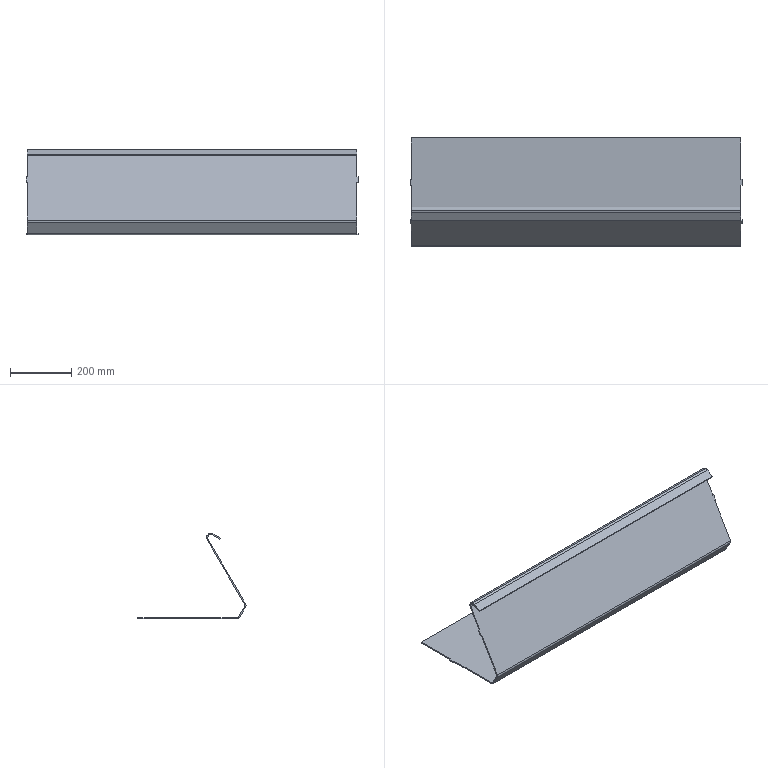Part | SolidWorks | features SM3dBend 3, FlatPattern 1, SMBaseFlange 1, SheetMetal 1 | 1 solid | 48 faces | box 1084 x 353.006 x 279.006 mm | volume 2939163 mm3 | plane 40 | cylinder 8 | commonest cylinder face diameters 10 x2 18 x2 20 x2 28 x2
STEP:
#1=CARTESIAN_POINT('',(1271.731,577.865,275.006));
#2=VERTEX_POINT('',#1);
#3=CARTESIAN_POINT('',(1271.731,570.865,273.13));
#4=VERTEX_POINT('',#3);
#5=CARTESIAN_POINT('',(1271.731,577.865,261.006));
#6=DIRECTION('',(1.,0.,0.));
#7=DIRECTION('',(0.,0.,1.));
#8=AXIS2_PLACEMENT_3D('',#5,#6,#7);
#9=CIRCLE('',#8,14.);
#10=EDGE_CURVE('',#2,#4,#9,.T.);
#11=ORIENTED_EDGE('',*,*,#10,.F.);
#12=CARTESIAN_POINT('',(195.731,577.865,275.006));
#13=VERTEX_POINT('',#12);
#14=CARTESIAN_POINT('',(1810.249,577.865,275.006));
#15=DIRECTION('',(-1.,0.,0.));
#16=VECTOR('',#15,1000.);
#17=LINE('',#14,#16);
#18=EDGE_CURVE('',#2,#13,#17,.T.);
#19=ORIENTED_EDGE('',*,*,#18,.T.);
#20=CARTESIAN_POINT('',(195.731,570.865,273.13));
#21=VERTEX_POINT('',#20);
#22=CARTESIAN_POINT('',(195.731,577.865,261.006));
#23=DIRECTION('',(-1.,0.,0.));
#24=DIRECTION('',(0.,0.,1.));
#25=AXIS2_PLACEMENT_3D('',#22,#23,#24);
#26=CIRCLE('',#25,14.);
#27=EDGE_CURVE('',#21,#13,#26,.T.);
#28=ORIENTED_EDGE('',*,*,#27,.F.);
#29=CARTESIAN_POINT('',(0.,570.865,273.13));
#30=DIRECTION('',(1.,0.,0.));
#31=VECTOR('',#30,1000.);
#32=LINE('',#29,#31);
#33=EDGE_CURVE('',#21,#4,#32,.T.);
#34=ORIENTED_EDGE('',*,*,#33,.T.);
#35=EDGE_LOOP('',(#11,#19,#28,#34));
#36=FACE_OUTER_BOUND('',#35,.T.);
#37=CARTESIAN_POINT('',(1810.249,577.865,261.006));
#38=DIRECTION('',(-1.,0.,0.));
#39=DIRECTION('',(0.,0.,1.));
#40=AXIS2_PLACEMENT_3D('',#37,#38,#39);
#41=CYLINDRICAL_SURFACE('',#40,14.);
#42=ADVANCED_FACE('',(#36),#41,.T.);
#43=CARTESIAN_POINT('',(1271.731,586.525,256.006));
#44=VERTEX_POINT('',#43);
#45=CARTESIAN_POINT('',(1271.731,577.865,271.006));
#46=VERTEX_POINT('',#45);
#47=CARTESIAN_POINT('',(1271.731,577.865,261.006));
#48=DIRECTION('',(1.,0.,0.));
#49=DIRECTION('',(0.,0.,1.));
#50=AXIS2_PLACEMENT_3D('',#47,#48,#49);
#51=CIRCLE('',#50,10.);
#52=EDGE_CURVE('',#44,#46,#51,.T.);
#53=ORIENTED_EDGE('',*,*,#52,.T.);
#54=CARTESIAN_POINT('',(195.731,577.865,271.006));
#55=VERTEX_POINT('',#54);
#56=CARTESIAN_POINT('',(1810.249,577.865,271.006));
#57=DIRECTION('',(-1.,0.,0.));
#58=VECTOR('',#57,1000.);
#59=LINE('',#56,#58);
#60=EDGE_CURVE('',#46,#55,#59,.T.);
#61=ORIENTED_EDGE('',*,*,#60,.T.);
#62=CARTESIAN_POINT('',(195.731,586.525,256.006));
#63=VERTEX_POINT('',#62);
#64=CARTESIAN_POINT('',(195.731,577.865,261.006));
#65=DIRECTION('',(-1.,0.,0.));
#66=DIRECTION('',(0.,0.,-1.));
#67=AXIS2_PLACEMENT_3D('',#64,#65,#66);
#68=CIRCLE('',#67,10.);
#69=EDGE_CURVE('',#55,#63,#68,.T.);
#70=ORIENTED_EDGE('',*,*,#69,.T.);
#71=CARTESIAN_POINT('',(0.,586.525,256.006));
#72=DIRECTION('',(1.,0.,0.));
#73=VECTOR('',#72,1000.);
#74=LINE('',#71,#73);
#75=EDGE_CURVE('',#63,#44,#74,.T.);
#76=ORIENTED_EDGE('',*,*,#75,.T.);
#77=EDGE_LOOP('',(#53,#61,#70,#76));
#78=FACE_OUTER_BOUND('',#77,.T.);
#79=CARTESIAN_POINT('',(1810.249,577.865,261.006));
#80=DIRECTION('',(-1.,0.,0.));
#81=DIRECTION('',(0.,0.,1.));
#82=AXIS2_PLACEMENT_3D('',#79,#80,#81);
#83=CYLINDRICAL_SURFACE('',#82,10.);
#84=ADVANCED_FACE('',(#78),#83,.F.);
#85=CARTESIAN_POINT('',(195.731,548.991,182.994));
#86=VERTEX_POINT('',#85);
#87=CARTESIAN_POINT('',(195.731,589.989,254.006));
#88=VERTEX_POINT('',#87);
#89=CARTESIAN_POINT('',(195.731,618.751,303.822));
#90=DIRECTION('',(0.,0.5,0.866));
#91=VECTOR('',#90,1000.);
#92=LINE('',#89,#91);
#93=EDGE_CURVE('',#86,#88,#92,.T.);
#94=ORIENTED_EDGE('',*,*,#93,.T.);
#95=CARTESIAN_POINT('',(1271.731,589.989,254.006));
#96=VERTEX_POINT('',#95);
#97=CARTESIAN_POINT('',(0.,589.989,254.006));
#98=DIRECTION('',(1.,0.,0.));
#99=VECTOR('',#98,1000.);
#100=LINE('',#97,#99);
#101=EDGE_CURVE('',#88,#96,#100,.T.);
#102=ORIENTED_EDGE('',*,*,#101,.T.);
#103=CARTESIAN_POINT('',(1271.731,548.991,182.994));
#104=VERTEX_POINT('',#103);
#105=CARTESIAN_POINT('',(1271.731,618.751,303.822));
#106=DIRECTION('',(0.,-0.5,-0.866));
#107=VECTOR('',#106,1000.);
#108=LINE('',#105,#107);
#109=EDGE_CURVE('',#96,#104,#108,.T.);
#110=ORIENTED_EDGE('',*,*,#109,.T.);
#111=CARTESIAN_POINT('',(1275.731,548.991,182.994));
#112=VERTEX_POINT('',#111);
#113=CARTESIAN_POINT('',(1275.731,548.991,182.994));
#114=DIRECTION('',(1.,0.,0.));
#115=VECTOR('',#114,1000.);
#116=LINE('',#113,#115);
#117=EDGE_CURVE('',#104,#112,#116,.T.);
#118=ORIENTED_EDGE('',*,*,#117,.T.);
#119=CARTESIAN_POINT('',(1275.731,538.991,165.674));
#120=VERTEX_POINT('',#119);
#121=CARTESIAN_POINT('',(1275.731,538.991,165.674));
#122=DIRECTION('',(0.,-0.5,-0.866));
#123=VECTOR('',#122,1000.);
#124=LINE('',#121,#123);
#125=EDGE_CURVE('',#112,#120,#124,.T.);
#126=ORIENTED_EDGE('',*,*,#125,.T.);
#127=CARTESIAN_POINT('',(1271.731,538.991,165.674));
#128=VERTEX_POINT('',#127);
#129=CARTESIAN_POINT('',(1275.731,538.991,165.674));
#130=DIRECTION('',(-1.,0.,0.));
#131=VECTOR('',#130,1000.);
#132=LINE('',#129,#131);
#133=EDGE_CURVE('',#120,#128,#132,.T.);
#134=ORIENTED_EDGE('',*,*,#133,.T.);
#135=CARTESIAN_POINT('',(1271.731,467.476,41.807));
#136=VERTEX_POINT('',#135);
#137=CARTESIAN_POINT('',(1271.731,538.991,165.674));
#138=DIRECTION('',(0.,-0.5,-0.866));
#139=VECTOR('',#138,1000.);
#140=LINE('',#137,#139);
#141=EDGE_CURVE('',#128,#136,#140,.T.);
#142=ORIENTED_EDGE('',*,*,#141,.T.);
#143=CARTESIAN_POINT('',(195.731,467.476,41.807));
#144=VERTEX_POINT('',#143);
#145=CARTESIAN_POINT('',(0.,467.476,41.807));
#146=DIRECTION('',(1.,0.,0.));
#147=VECTOR('',#146,1000.);
#148=LINE('',#145,#147);
#149=EDGE_CURVE('',#144,#136,#148,.T.);
#150=ORIENTED_EDGE('',*,*,#149,.F.);
#151=CARTESIAN_POINT('',(195.731,538.991,165.674));
#152=VERTEX_POINT('',#151);
#153=CARTESIAN_POINT('',(195.731,538.991,165.674));
#154=DIRECTION('',(0.,0.5,0.866));
#155=VECTOR('',#154,1000.);
#156=LINE('',#153,#155);
#157=EDGE_CURVE('',#144,#152,#156,.T.);
#158=ORIENTED_EDGE('',*,*,#157,.T.);
#159=CARTESIAN_POINT('',(191.731,538.991,165.674));
#160=VERTEX_POINT('',#159);
#161=CARTESIAN_POINT('',(191.731,538.991,165.674));
#162=DIRECTION('',(-1.,0.,0.));
#163=VECTOR('',#162,1000.);
#164=LINE('',#161,#163);
#165=EDGE_CURVE('',#152,#160,#164,.T.);
#166=ORIENTED_EDGE('',*,*,#165,.T.);
#167=CARTESIAN_POINT('',(191.731,548.991,182.994));
#168=VERTEX_POINT('',#167);
#169=CARTESIAN_POINT('',(191.731,548.991,182.994));
#170=DIRECTION('',(0.,0.5,0.866));
#171=VECTOR('',#170,1000.);
#172=LINE('',#169,#171);
#173=EDGE_CURVE('',#160,#168,#172,.T.);
#174=ORIENTED_EDGE('',*,*,#173,.T.);
#175=CARTESIAN_POINT('',(191.731,548.991,182.994));
#176=DIRECTION('',(1.,0.,0.));
#177=VECTOR('',#176,1000.);
#178=LINE('',#175,#177);
#179=EDGE_CURVE('',#168,#86,#178,.T.);
#180=ORIENTED_EDGE('',*,*,#179,.T.);
#181=EDGE_LOOP('',(#94,#102,#110,#118,#126,#134,#142,#150,#158,#166,#174,#180));
#182=FACE_OUTER_BOUND('',#181,.T.);
#183=CARTESIAN_POINT('',(0.,686.774,421.641));
#184=DIRECTION('',(0.,-0.866,0.5));
#185=DIRECTION('',(-1.,0.,0.));
#186=AXIS2_PLACEMENT_3D('',#183,#184,#185);
#187=PLANE('',#186);
#188=ADVANCED_FACE('',(#182),#187,.F.);
#189=CARTESIAN_POINT('',(195.731,487.283,2.5));
#190=VERTEX_POINT('',#189);
#191=CARTESIAN_POINT('',(195.731,467.476,36.807));
#192=VERTEX_POINT('',#191);
#193=CARTESIAN_POINT('',(195.731,392.611,166.478));
#194=DIRECTION('',(0.,-0.5,0.866));
#195=VECTOR('',#194,1000.);
#196=LINE('',#193,#195);
#197=EDGE_CURVE('',#190,#192,#196,.T.);
#198=ORIENTED_EDGE('',*,*,#197,.T.);
#199=CARTESIAN_POINT('',(1271.731,467.476,36.807));
#200=VERTEX_POINT('',#199);
#201=CARTESIAN_POINT('',(0.,467.476,36.807));
#202=DIRECTION('',(1.,0.,0.));
#203=VECTOR('',#202,1000.);
#204=LINE('',#201,#203);
#205=EDGE_CURVE('',#192,#200,#204,.T.);
#206=ORIENTED_EDGE('',*,*,#205,.T.);
#207=CARTESIAN_POINT('',(1271.731,487.283,2.5));
#208=VERTEX_POINT('',#207);
#209=CARTESIAN_POINT('',(1271.731,392.611,166.478));
#210=DIRECTION('',(0.,0.5,-0.866));
#211=VECTOR('',#210,1000.);
#212=LINE('',#209,#211);
#213=EDGE_CURVE('',#200,#208,#212,.T.);
#214=ORIENTED_EDGE('',*,*,#213,.T.);
#215=CARTESIAN_POINT('',(0.,487.283,2.5));
#216=DIRECTION('',(1.,0.,0.));
#217=VECTOR('',#216,1000.);
#218=LINE('',#215,#217);
#219=EDGE_CURVE('',#190,#208,#218,.T.);
#220=ORIENTED_EDGE('',*,*,#219,.F.);
#221=EDGE_LOOP('',(#198,#206,#214,#220));
#222=FACE_OUTER_BOUND('',#221,.T.);
#223=CARTESIAN_POINT('',(0.,244.828,422.446));
#224=DIRECTION('',(0.,-0.866,-0.5));
#225=DIRECTION('',(-1.,0.,0.));
#226=AXIS2_PLACEMENT_3D('',#223,#224,#225);
#227=PLANE('',#226);
#228=ADVANCED_FACE('',(#222),#227,.F.);
#229=CARTESIAN_POINT('',(195.731,464.012,34.807));
#230=VERTEX_POINT('',#229);
#231=CARTESIAN_POINT('',(195.731,464.012,34.807));
#232=DIRECTION('',(0.,-0.866,-0.5));
#233=VECTOR('',#232,1000.);
#234=LINE('',#231,#233);
#235=EDGE_CURVE('',#192,#230,#234,.T.);
#236=ORIENTED_EDGE('',*,*,#235,.F.);
#237=ORIENTED_EDGE('',*,*,#197,.F.);
#238=CARTESIAN_POINT('',(195.731,483.819,0.5));
#239=VERTEX_POINT('',#238);
#240=CARTESIAN_POINT('',(195.731,483.819,0.5));
#241=DIRECTION('',(0.,-0.866,-0.5));
#242=VECTOR('',#241,1000.);
#243=LINE('',#240,#242);
#244=EDGE_CURVE('',#190,#239,#243,.T.);
#245=ORIENTED_EDGE('',*,*,#244,.T.);
#246=CARTESIAN_POINT('',(195.731,389.147,164.478));
#247=DIRECTION('',(0.,-0.5,0.866));
#248=VECTOR('',#247,1000.);
#249=LINE('',#246,#248);
#250=EDGE_CURVE('',#239,#230,#249,.T.);
#251=ORIENTED_EDGE('',*,*,#250,.T.);
#252=EDGE_LOOP('',(#236,#237,#245,#251));
#253=FACE_OUTER_BOUND('',#252,.T.);
#254=CARTESIAN_POINT('',(195.731,389.147,164.478));
#255=DIRECTION('',(-1.,0.,0.));
#256=DIRECTION('',(0.,0.866,0.5));
#257=AXIS2_PLACEMENT_3D('',#254,#255,#256);
#258=PLANE('',#257);
#259=ADVANCED_FACE('',(#253),#258,.T.);
#260=CARTESIAN_POINT('',(1271.731,464.012,34.807));
#261=VERTEX_POINT('',#260);
#262=CARTESIAN_POINT('',(1271.731,464.012,34.807));
#263=DIRECTION('',(0.,0.866,0.5));
#264=VECTOR('',#263,1000.);
#265=LINE('',#262,#264);
#266=EDGE_CURVE('',#261,#200,#265,.T.);
#267=ORIENTED_EDGE('',*,*,#266,.F.);
#268=CARTESIAN_POINT('',(1271.731,483.819,0.5));
#269=VERTEX_POINT('',#268);
#270=CARTESIAN_POINT('',(1271.731,389.147,164.478));
#271=DIRECTION('',(0.,0.5,-0.866));
#272=VECTOR('',#271,1000.);
#273=LINE('',#270,#272);
#274=EDGE_CURVE('',#261,#269,#273,.T.);
#275=ORIENTED_EDGE('',*,*,#274,.T.);
#276=CARTESIAN_POINT('',(1271.731,483.819,0.5));
#277=DIRECTION('',(0.,0.866,0.5));
#278=VECTOR('',#277,1000.);
#279=LINE('',#276,#278);
#280=EDGE_CURVE('',#269,#208,#279,.T.);
#281=ORIENTED_EDGE('',*,*,#280,.T.);
#282=ORIENTED_EDGE('',*,*,#213,.F.);
#283=EDGE_LOOP('',(#267,#275,#281,#282));
#284=FACE_OUTER_BOUND('',#283,.T.);
#285=CARTESIAN_POINT('',(1271.731,389.147,164.478));
#286=DIRECTION('',(1.,0.,0.));
#287=DIRECTION('',(0.,-0.866,-0.5));
#288=AXIS2_PLACEMENT_3D('',#285,#286,#287);
#289=PLANE('',#288);
#290=ADVANCED_FACE('',(#284),#289,.T.);
#291=CARTESIAN_POINT('',(0.,464.012,34.807));
#292=DIRECTION('',(1.,0.,0.));
#293=VECTOR('',#292,1000.);
#294=LINE('',#291,#293);
#295=EDGE_CURVE('',#230,#261,#294,.T.);
#296=ORIENTED_EDGE('',*,*,#295,.F.);
#297=ORIENTED_EDGE('',*,*,#250,.F.);
#298=CARTESIAN_POINT('',(0.,483.819,0.5));
#299=DIRECTION('',(1.,0.,0.));
#300=VECTOR('',#299,1000.);
#301=LINE('',#298,#300);
#302=EDGE_CURVE('',#239,#269,#301,.T.);
#303=ORIENTED_EDGE('',*,*,#302,.T.);
#304=ORIENTED_EDGE('',*,*,#274,.F.);
#305=EDGE_LOOP('',(#296,#297,#303,#304));
#306=FACE_OUTER_BOUND('',#305,.T.);
#307=CARTESIAN_POINT('',(0.,241.363,420.446));
#308=DIRECTION('',(0.,-0.866,-0.5));
#309=DIRECTION('',(-1.,0.,0.));
#310=AXIS2_PLACEMENT_3D('',#307,#308,#309);
#311=PLANE('',#310);
#312=ADVANCED_FACE('',(#306),#311,.T.);
#313=CARTESIAN_POINT('',(1271.731,660.806,0.));
#314=VERTEX_POINT('',#313);
#315=CARTESIAN_POINT('',(1275.731,660.806,0.));
#316=VERTEX_POINT('',#315);
#317=CARTESIAN_POINT('',(1275.731,660.806,0.));
#318=DIRECTION('',(1.,0.,0.));
#319=VECTOR('',#318,1000.);
#320=LINE('',#317,#319);
#321=EDGE_CURVE('',#314,#316,#320,.T.);
#322=ORIENTED_EDGE('',*,*,#321,.F.);
#323=CARTESIAN_POINT('',(1271.731,660.806,-4.));
#324=VERTEX_POINT('',#323);
#325=CARTESIAN_POINT('',(1271.731,660.806,-4.));
#326=DIRECTION('',(0.,0.,1.));
#327=VECTOR('',#326,1000.);
#328=LINE('',#325,#327);
#329=EDGE_CURVE('',#324,#314,#328,.T.);
#330=ORIENTED_EDGE('',*,*,#329,.F.);
#331=CARTESIAN_POINT('',(1275.731,660.806,-4.));
#332=VERTEX_POINT('',#331);
#333=CARTESIAN_POINT('',(1275.731,660.806,-4.));
#334=DIRECTION('',(1.,0.,0.));
#335=VECTOR('',#334,1000.);
#336=LINE('',#333,#335);
#337=EDGE_CURVE('',#324,#332,#336,.T.);
#338=ORIENTED_EDGE('',*,*,#337,.T.);
#339=CARTESIAN_POINT('',(1275.731,660.806,-4.));
#340=DIRECTION('',(0.,0.,1.));
#341=VECTOR('',#340,1000.);
#342=LINE('',#339,#341);
#343=EDGE_CURVE('',#332,#316,#342,.T.);
#344=ORIENTED_EDGE('',*,*,#343,.T.);
#345=EDGE_LOOP('',(#322,#330,#338,#344));
#346=FACE_OUTER_BOUND('',#345,.T.);
#347=CARTESIAN_POINT('',(1275.731,660.806,-4.));
#348=DIRECTION('',(0.,-1.,0.));
#349=DIRECTION('',(0.,0.,-1.));
#350=AXIS2_PLACEMENT_3D('',#347,#348,#349);
#351=PLANE('',#350);
#352=ADVANCED_FACE('',(#346),#351,.T.);
#353=CARTESIAN_POINT('',(1275.731,680.806,0.));
#354=VERTEX_POINT('',#353);
#355=CARTESIAN_POINT('',(1275.731,680.806,0.));
#356=DIRECTION('',(0.,1.,0.));
#357=VECTOR('',#356,1000.);
#358=LINE('',#355,#357);
#359=EDGE_CURVE('',#316,#354,#358,.T.);
#360=ORIENTED_EDGE('',*,*,#359,.F.);
#361=ORIENTED_EDGE('',*,*,#343,.F.);
#362=CARTESIAN_POINT('',(1275.731,680.806,-4.));
#363=VERTEX_POINT('',#362);
#364=CARTESIAN_POINT('',(1275.731,680.806,-4.));
#365=DIRECTION('',(0.,1.,0.));
#366=VECTOR('',#365,1000.);
#367=LINE('',#364,#366);
#368=EDGE_CURVE('',#332,#363,#367,.T.);
#369=ORIENTED_EDGE('',*,*,#368,.T.);
#370=CARTESIAN_POINT('',(1275.731,680.806,-4.));
#371=DIRECTION('',(0.,0.,1.));
#372=VECTOR('',#371,1000.);
#373=LINE('',#370,#372);
#374=EDGE_CURVE('',#363,#354,#373,.T.);
#375=ORIENTED_EDGE('',*,*,#374,.T.);
#376=EDGE_LOOP('',(#360,#361,#369,#375));
#377=FACE_OUTER_BOUND('',#376,.T.);
#378=CARTESIAN_POINT('',(1275.731,680.806,-4.));
#379=DIRECTION('',(1.,0.,0.));
#380=DIRECTION('',(0.,0.,-1.));
#381=AXIS2_PLACEMENT_3D('',#378,#379,#380);
#382=PLANE('',#381);
#383=ADVANCED_FACE('',(#377),#382,.T.);
#384=CARTESIAN_POINT('',(1271.731,680.806,0.));
#385=VERTEX_POINT('',#384);
#386=CARTESIAN_POINT('',(1275.731,680.806,0.));
#387=DIRECTION('',(-1.,0.,0.));
#388=VECTOR('',#387,1000.);
#389=LINE('',#386,#388);
#390=EDGE_CURVE('',#354,#385,#389,.T.);
#391=ORIENTED_EDGE('',*,*,#390,.F.);
#392=ORIENTED_EDGE('',*,*,#374,.F.);
#393=CARTESIAN_POINT('',(1271.731,680.806,-4.));
#394=VERTEX_POINT('',#393);
#395=CARTESIAN_POINT('',(1275.731,680.806,-4.));
#396=DIRECTION('',(-1.,0.,0.));
#397=VECTOR('',#396,1000.);
#398=LINE('',#395,#397);
#399=EDGE_CURVE('',#363,#394,#398,.T.);
#400=ORIENTED_EDGE('',*,*,#399,.T.);
#401=CARTESIAN_POINT('',(1271.731,680.806,-4.));
#402=DIRECTION('',(0.,0.,1.));
#403=VECTOR('',#402,1000.);
#404=LINE('',#401,#403);
#405=EDGE_CURVE('',#394,#385,#404,.T.);
#406=ORIENTED_EDGE('',*,*,#405,.T.);
#407=EDGE_LOOP('',(#391,#392,#400,#406));
#408=FACE_OUTER_BOUND('',#407,.T.);
#409=CARTESIAN_POINT('',(1275.731,680.806,-4.));
#410=DIRECTION('',(0.,1.,0.));
#411=DIRECTION('',(0.,0.,1.));
#412=AXIS2_PLACEMENT_3D('',#409,#410,#411);
#413=PLANE('',#412);
#414=ADVANCED_FACE('',(#408),#413,.T.);
#415=CARTESIAN_POINT('',(1271.731,815.812,0.));
#416=VERTEX_POINT('',#415);
#417=CARTESIAN_POINT('',(1271.731,680.806,0.));
#418=DIRECTION('',(0.,1.,0.));
#419=VECTOR('',#418,1000.);
#420=LINE('',#417,#419);
#421=EDGE_CURVE('',#385,#416,#420,.T.);
#422=ORIENTED_EDGE('',*,*,#421,.F.);
#423=ORIENTED_EDGE('',*,*,#405,.F.);
#424=CARTESIAN_POINT('',(1271.731,815.812,-4.));
#425=VERTEX_POINT('',#424);
#426=CARTESIAN_POINT('',(1271.731,680.806,-4.));
#427=DIRECTION('',(0.,1.,0.));
#428=VECTOR('',#427,1000.);
#429=LINE('',#426,#428);
#430=EDGE_CURVE('',#394,#425,#429,.T.);
#431=ORIENTED_EDGE('',*,*,#430,.T.);
#432=CARTESIAN_POINT('',(1271.731,815.812,-4.));
#433=DIRECTION('',(0.,0.,1.));
#434=VECTOR('',#433,1000.);
#435=LINE('',#432,#434);
#436=EDGE_CURVE('',#425,#416,#435,.T.);
#437=ORIENTED_EDGE('',*,*,#436,.T.);
#438=EDGE_LOOP('',(#422,#423,#431,#437));
#439=FACE_OUTER_BOUND('',#438,.T.);
#440=CARTESIAN_POINT('',(1271.731,680.806,-4.));
#441=DIRECTION('',(1.,0.,0.));
#442=DIRECTION('',(0.,0.,-1.));
#443=AXIS2_PLACEMENT_3D('',#440,#441,#442);
#444=PLANE('',#443);
#445=ADVANCED_FACE('',(#439),#444,.T.);
#446=CARTESIAN_POINT('',(195.731,815.812,0.));
#447=VERTEX_POINT('',#446);
#448=CARTESIAN_POINT('',(1271.731,815.812,0.));
#449=DIRECTION('',(-1.,0.,0.));
#450=VECTOR('',#449,1000.);
#451=LINE('',#448,#450);
#452=EDGE_CURVE('',#416,#447,#451,.T.);
#453=ORIENTED_EDGE('',*,*,#452,.F.);
#454=ORIENTED_EDGE('',*,*,#436,.F.);
#455=CARTESIAN_POINT('',(195.731,815.812,-4.));
#456=VERTEX_POINT('',#455);
#457=CARTESIAN_POINT('',(1271.731,815.812,-4.));
#458=DIRECTION('',(-1.,0.,0.));
#459=VECTOR('',#458,1000.);
#460=LINE('',#457,#459);
#461=EDGE_CURVE('',#425,#456,#460,.T.);
#462=ORIENTED_EDGE('',*,*,#461,.T.);
#463=CARTESIAN_POINT('',(195.731,815.812,-4.));
#464=DIRECTION('',(0.,0.,1.));
#465=VECTOR('',#464,1000.);
#466=LINE('',#463,#465);
#467=EDGE_CURVE('',#456,#447,#466,.T.);
#468=ORIENTED_EDGE('',*,*,#467,.T.);
#469=EDGE_LOOP('',(#453,#454,#462,#468));
#470=FACE_OUTER_BOUND('',#469,.T.);
#471=CARTESIAN_POINT('',(1271.731,815.812,-4.));
#472=DIRECTION('',(0.,1.,0.));
#473=DIRECTION('',(-1.,0.,0.));
#474=AXIS2_PLACEMENT_3D('',#471,#472,#473);
#475=PLANE('',#474);
#476=ADVANCED_FACE('',(#470),#475,.T.);
#477=CARTESIAN_POINT('',(195.731,680.806,0.));
#478=VERTEX_POINT('',#477);
#479=CARTESIAN_POINT('',(195.731,680.806,0.));
#480=DIRECTION('',(0.,-1.,0.));
#481=VECTOR('',#480,1000.);
#482=LINE('',#479,#481);
#483=EDGE_CURVE('',#447,#478,#482,.T.);
#484=ORIENTED_EDGE('',*,*,#483,.F.);
#485=ORIENTED_EDGE('',*,*,#467,.F.);
#486=CARTESIAN_POINT('',(195.731,680.806,-4.));
#487=VERTEX_POINT('',#486);
#488=CARTESIAN_POINT('',(195.731,680.806,-4.));
#489=DIRECTION('',(0.,-1.,0.));
#490=VECTOR('',#489,1000.);
#491=LINE('',#488,#490);
#492=EDGE_CURVE('',#456,#487,#491,.T.);
#493=ORIENTED_EDGE('',*,*,#492,.T.);
#494=CARTESIAN_POINT('',(195.731,680.806,-4.));
#495=DIRECTION('',(0.,0.,1.));
#496=VECTOR('',#495,1000.);
#497=LINE('',#494,#496);
#498=EDGE_CURVE('',#487,#478,#497,.T.);
#499=ORIENTED_EDGE('',*,*,#498,.T.);
#500=EDGE_LOOP('',(#484,#485,#493,#499));
#501=FACE_OUTER_BOUND('',#500,.T.);
#502=CARTESIAN_POINT('',(195.731,680.806,-4.));
#503=DIRECTION('',(-1.,0.,0.));
#504=DIRECTION('',(0.,0.,1.));
#505=AXIS2_PLACEMENT_3D('',#502,#503,#504);
#506=PLANE('',#505);
#507=ADVANCED_FACE('',(#501),#506,.T.);
#508=CARTESIAN_POINT('',(191.731,680.806,0.));
#509=VERTEX_POINT('',#508);
#510=CARTESIAN_POINT('',(191.731,680.806,0.));
#511=DIRECTION('',(-1.,0.,0.));
#512=VECTOR('',#511,1000.);
#513=LINE('',#510,#512);
#514=EDGE_CURVE('',#478,#509,#513,.T.);
#515=ORIENTED_EDGE('',*,*,#514,.F.);
#516=ORIENTED_EDGE('',*,*,#498,.F.);
#517=CARTESIAN_POINT('',(191.731,680.806,-4.));
#518=VERTEX_POINT('',#517);
#519=CARTESIAN_POINT('',(191.731,680.806,-4.));
#520=DIRECTION('',(-1.,0.,0.));
#521=VECTOR('',#520,1000.);
#522=LINE('',#519,#521);
#523=EDGE_CURVE('',#487,#518,#522,.T.);
#524=ORIENTED_EDGE('',*,*,#523,.T.);
#525=CARTESIAN_POINT('',(191.731,680.806,-4.));
#526=DIRECTION('',(0.,0.,1.));
#527=VECTOR('',#526,1000.);
#528=LINE('',#525,#527);
#529=EDGE_CURVE('',#518,#509,#528,.T.);
#530=ORIENTED_EDGE('',*,*,#529,.T.);
#531=EDGE_LOOP('',(#515,#516,#524,#530));
#532=FACE_OUTER_BOUND('',#531,.T.);
#533=CARTESIAN_POINT('',(191.731,680.806,-4.));
#534=DIRECTION('',(0.,1.,0.));
#535=DIRECTION('',(0.,0.,1.));
#536=AXIS2_PLACEMENT_3D('',#533,#534,#535);
#537=PLANE('',#536);
#538=ADVANCED_FACE('',(#532),#537,.T.);
#539=CARTESIAN_POINT('',(191.731,660.806,0.));
#540=VERTEX_POINT('',#539);
#541=CARTESIAN_POINT('',(191.731,660.806,0.));
#542=DIRECTION('',(0.,-1.,0.));
#543=VECTOR('',#542,1000.);
#544=LINE('',#541,#543);
#545=EDGE_CURVE('',#509,#540,#544,.T.);
#546=ORIENTED_EDGE('',*,*,#545,.F.);
#547=ORIENTED_EDGE('',*,*,#529,.F.);
#548=CARTESIAN_POINT('',(191.731,660.806,-4.));
#549=VERTEX_POINT('',#548);
#550=CARTESIAN_POINT('',(191.731,660.806,-4.));
#551=DIRECTION('',(0.,-1.,0.));
#552=VECTOR('',#551,1000.);
#553=LINE('',#550,#552);
#554=EDGE_CURVE('',#518,#549,#553,.T.);
#555=ORIENTED_EDGE('',*,*,#554,.T.);
#556=CARTESIAN_POINT('',(191.731,660.806,-4.));
#557=DIRECTION('',(0.,0.,1.));
#558=VECTOR('',#557,1000.);
#559=LINE('',#556,#558);
#560=EDGE_CURVE('',#549,#540,#559,.T.);
#561=ORIENTED_EDGE('',*,*,#560,.T.);
#562=EDGE_LOOP('',(#546,#547,#555,#561));
#563=FACE_OUTER_BOUND('',#562,.T.);
#564=CARTESIAN_POINT('',(191.731,660.806,-4.));
#565=DIRECTION('',(-1.,0.,0.));
#566=DIRECTION('',(0.,0.,1.));
#567=AXIS2_PLACEMENT_3D('',#564,#565,#566);
#568=PLANE('',#567);
#569=ADVANCED_FACE('',(#563),#568,.T.);
#570=CARTESIAN_POINT('',(195.731,660.806,0.));
#571=VERTEX_POINT('',#570);
#572=CARTESIAN_POINT('',(191.731,660.806,0.));
#573=DIRECTION('',(1.,0.,0.));
#574=VECTOR('',#573,1000.);
#575=LINE('',#572,#574);
#576=EDGE_CURVE('',#540,#571,#575,.T.);
#577=ORIENTED_EDGE('',*,*,#576,.F.);
#578=ORIENTED_EDGE('',*,*,#560,.F.);
#579=CARTESIAN_POINT('',(195.731,660.806,-4.));
#580=VERTEX_POINT('',#579);
#581=CARTESIAN_POINT('',(191.731,660.806,-4.));
#582=DIRECTION('',(1.,0.,0.));
#583=VECTOR('',#582,1000.);
#584=LINE('',#581,#583);
#585=EDGE_CURVE('',#549,#580,#584,.T.);
#586=ORIENTED_EDGE('',*,*,#585,.T.);
#587=CARTESIAN_POINT('',(195.731,660.806,-4.));
#588=DIRECTION('',(0.,0.,1.));
#589=VECTOR('',#588,1000.);
#590=LINE('',#587,#589);
#591=EDGE_CURVE('',#580,#571,#590,.T.);
#592=ORIENTED_EDGE('',*,*,#591,.T.);
#593=EDGE_LOOP('',(#577,#578,#586,#592));
#594=FACE_OUTER_BOUND('',#593,.T.);
#595=CARTESIAN_POINT('',(191.731,660.806,-4.));
#596=DIRECTION('',(0.,-1.,0.));
#597=DIRECTION('',(0.,0.,-1.));
#598=AXIS2_PLACEMENT_3D('',#595,#596,#597);
#599=PLANE('',#598);
#600=ADVANCED_FACE('',(#594),#599,.T.);
#601=CARTESIAN_POINT('',(195.731,491.613,-4.));
#602=VERTEX_POINT('',#601);
#603=CARTESIAN_POINT('',(1271.731,491.613,-4.));
#604=VERTEX_POINT('',#603);
#605=CARTESIAN_POINT('',(0.,491.613,-4.));
#606=DIRECTION('',(1.,0.,0.));
#607=VECTOR('',#606,1000.);
#608=LINE('',#605,#607);
#609=EDGE_CURVE('',#602,#604,#608,.T.);
#610=ORIENTED_EDGE('',*,*,#609,.F.);
#611=CARTESIAN_POINT('',(195.731,295.566,-4.));
#612=DIRECTION('',(0.,-1.,0.));
#613=VECTOR('',#612,1000.);
#614=LINE('',#611,#613);
#615=EDGE_CURVE('',#580,#602,#614,.T.);
#616=ORIENTED_EDGE('',*,*,#615,.F.);
#617=ORIENTED_EDGE('',*,*,#585,.F.);
#618=ORIENTED_EDGE('',*,*,#554,.F.);
#619=ORIENTED_EDGE('',*,*,#523,.F.);
#620=ORIENTED_EDGE('',*,*,#492,.F.);
#621=ORIENTED_EDGE('',*,*,#461,.F.);
#622=ORIENTED_EDGE('',*,*,#430,.F.);
#623=ORIENTED_EDGE('',*,*,#399,.F.);
#624=ORIENTED_EDGE('',*,*,#368,.F.);
#625=ORIENTED_EDGE('',*,*,#337,.F.);
#626=CARTESIAN_POINT('',(1271.731,295.566,-4.));
#627=DIRECTION('',(0.,1.,0.));
#628=VECTOR('',#627,1000.);
#629=LINE('',#626,#628);
#630=EDGE_CURVE('',#604,#324,#629,.T.);
#631=ORIENTED_EDGE('',*,*,#630,.F.);
#632=EDGE_LOOP('',(#610,#616,#617,#618,#619,#620,#621,#622,#623,#624,#625,#631));
#633=FACE_OUTER_BOUND('',#632,.T.);
#634=CARTESIAN_POINT('',(0.,0.,-4.));
#635=DIRECTION('',(0.,0.,-1.));
#636=DIRECTION('',(-1.,0.,0.));
#637=AXIS2_PLACEMENT_3D('',#634,#635,#636);
#638=PLANE('',#637);
#639=ADVANCED_FACE('',(#633),#638,.T.);
#640=CARTESIAN_POINT('',(195.731,491.613,0.));
#641=VERTEX_POINT('',#640);
#642=CARTESIAN_POINT('',(195.731,491.613,-4.));
#643=DIRECTION('',(0.,0.,-1.));
#644=VECTOR('',#643,1000.);
#645=LINE('',#642,#644);
#646=EDGE_CURVE('',#641,#602,#645,.T.);
#647=ORIENTED_EDGE('',*,*,#646,.F.);
#648=CARTESIAN_POINT('',(195.731,295.566,0.));
#649=DIRECTION('',(0.,-1.,0.));
#650=VECTOR('',#649,1000.);
#651=LINE('',#648,#650);
#652=EDGE_CURVE('',#571,#641,#651,.T.);
#653=ORIENTED_EDGE('',*,*,#652,.F.);
#654=ORIENTED_EDGE('',*,*,#591,.F.);
#655=ORIENTED_EDGE('',*,*,#615,.T.);
#656=EDGE_LOOP('',(#647,#653,#654,#655));
#657=FACE_OUTER_BOUND('',#656,.T.);
#658=CARTESIAN_POINT('',(195.731,295.566,-4.));
#659=DIRECTION('',(-1.,0.,0.));
#660=DIRECTION('',(0.,0.,1.));
#661=AXIS2_PLACEMENT_3D('',#658,#659,#660);
#662=PLANE('',#661);
#663=ADVANCED_FACE('',(#657),#662,.T.);
#664=ORIENTED_EDGE('',*,*,#652,.T.);
#665=CARTESIAN_POINT('',(1271.731,491.613,0.));
#666=VERTEX_POINT('',#665);
#667=CARTESIAN_POINT('',(0.,491.613,0.));
#668=DIRECTION('',(1.,0.,0.));
#669=VECTOR('',#668,1000.);
#670=LINE('',#667,#669);
#671=EDGE_CURVE('',#641,#666,#670,.T.);
#672=ORIENTED_EDGE('',*,*,#671,.T.);
#673=CARTESIAN_POINT('',(1271.731,295.566,0.));
#674=DIRECTION('',(0.,1.,0.));
#675=VECTOR('',#674,1000.);
#676=LINE('',#673,#675);
#677=EDGE_CURVE('',#666,#314,#676,.T.);
#678=ORIENTED_EDGE('',*,*,#677,.T.);
#679=ORIENTED_EDGE('',*,*,#321,.T.);
#680=ORIENTED_EDGE('',*,*,#359,.T.);
#681=ORIENTED_EDGE('',*,*,#390,.T.);
#682=ORIENTED_EDGE('',*,*,#421,.T.);
#683=ORIENTED_EDGE('',*,*,#452,.T.);
#684=ORIENTED_EDGE('',*,*,#483,.T.);
#685=ORIENTED_EDGE('',*,*,#514,.T.);
#686=ORIENTED_EDGE('',*,*,#545,.T.);
#687=ORIENTED_EDGE('',*,*,#576,.T.);
#688=EDGE_LOOP('',(#664,#672,#678,#679,#680,#681,#682,#683,#684,#685,#686,#687));
#689=FACE_OUTER_BOUND('',#688,.T.);
#690=CARTESIAN_POINT('',(0.,0.,0.));
#691=DIRECTION('',(0.,0.,-1.));
#692=DIRECTION('',(-1.,0.,0.));
#693=AXIS2_PLACEMENT_3D('',#690,#691,#692);
#694=PLANE('',#693);
#695=ADVANCED_FACE('',(#689),#694,.F.);
#696=CARTESIAN_POINT('',(1271.731,491.613,-4.));
#697=DIRECTION('',(0.,0.,1.));
#698=VECTOR('',#697,1000.);
#699=LINE('',#696,#698);
#700=EDGE_CURVE('',#604,#666,#699,.T.);
#701=ORIENTED_EDGE('',*,*,#700,.F.);
#702=ORIENTED_EDGE('',*,*,#630,.T.);
#703=ORIENTED_EDGE('',*,*,#329,.T.);
#704=ORIENTED_EDGE('',*,*,#677,.F.);
#705=EDGE_LOOP('',(#701,#702,#703,#704));
#706=FACE_OUTER_BOUND('',#705,.T.);
#707=CARTESIAN_POINT('',(1271.731,295.566,-4.));
#708=DIRECTION('',(1.,0.,0.));
#709=DIRECTION('',(0.,0.,-1.));
#710=AXIS2_PLACEMENT_3D('',#707,#708,#709);
#711=PLANE('',#710);
#712=ADVANCED_FACE('',(#706),#711,.T.);
#713=ORIENTED_EDGE('',*,*,#244,.F.);
#714=CARTESIAN_POINT('',(195.731,491.613,5.));
#715=DIRECTION('',(1.,0.,0.));
#716=DIRECTION('',(0.,0.,1.));
#717=AXIS2_PLACEMENT_3D('',#714,#715,#716);
#718=CIRCLE('',#717,5.);
#719=EDGE_CURVE('',#190,#641,#718,.T.);
#720=ORIENTED_EDGE('',*,*,#719,.T.);
#721=ORIENTED_EDGE('',*,*,#646,.T.);
#722=CARTESIAN_POINT('',(195.731,491.613,5.));
#723=DIRECTION('',(1.,0.,0.));
#724=DIRECTION('',(0.,0.,1.));
#725=AXIS2_PLACEMENT_3D('',#722,#723,#724);
#726=CIRCLE('',#725,9.);
#727=EDGE_CURVE('',#239,#602,#726,.T.);
#728=ORIENTED_EDGE('',*,*,#727,.F.);
#729=EDGE_LOOP('',(#713,#720,#721,#728));
#730=FACE_OUTER_BOUND('',#729,.T.);
#731=CARTESIAN_POINT('',(195.731,491.613,5.));
#732=DIRECTION('',(-1.,0.,0.));
#733=DIRECTION('',(0.,0.,1.));
#734=AXIS2_PLACEMENT_3D('',#731,#732,#733);
#735=PLANE('',#734);
#736=ADVANCED_FACE('',(#730),#735,.T.);
#737=CARTESIAN_POINT('',(1271.731,491.613,5.));
#738=DIRECTION('',(-1.,0.,0.));
#739=DIRECTION('',(0.,0.,1.));
#740=AXIS2_PLACEMENT_3D('',#737,#738,#739);
#741=CIRCLE('',#740,5.);
#742=EDGE_CURVE('',#666,#208,#741,.T.);
#743=ORIENTED_EDGE('',*,*,#742,.T.);
#744=ORIENTED_EDGE('',*,*,#280,.F.);
#745=CARTESIAN_POINT('',(1271.731,491.613,5.));
#746=DIRECTION('',(-1.,0.,0.));
#747=DIRECTION('',(0.,0.,-1.));
#748=AXIS2_PLACEMENT_3D('',#745,#746,#747);
#749=CIRCLE('',#748,9.);
#750=EDGE_CURVE('',#604,#269,#749,.T.);
#751=ORIENTED_EDGE('',*,*,#750,.F.);
#752=ORIENTED_EDGE('',*,*,#700,.T.);
#753=EDGE_LOOP('',(#743,#744,#751,#752));
#754=FACE_OUTER_BOUND('',#753,.T.);
#755=CARTESIAN_POINT('',(1271.731,491.613,5.));
#756=DIRECTION('',(1.,0.,0.));
#757=DIRECTION('',(0.,0.,-1.));
#758=AXIS2_PLACEMENT_3D('',#755,#756,#757);
#759=PLANE('',#758);
#760=ADVANCED_FACE('',(#754),#759,.T.);
#761=ORIENTED_EDGE('',*,*,#609,.T.);
#762=ORIENTED_EDGE('',*,*,#750,.T.);
#763=ORIENTED_EDGE('',*,*,#302,.F.);
#764=ORIENTED_EDGE('',*,*,#727,.T.);
#765=EDGE_LOOP('',(#761,#762,#763,#764));
#766=FACE_OUTER_BOUND('',#765,.T.);
#767=CARTESIAN_POINT('',(1809.76,491.613,5.));
#768=DIRECTION('',(-1.,0.,0.));
#769=DIRECTION('',(0.,0.,1.));
#770=AXIS2_PLACEMENT_3D('',#767,#768,#769);
#771=CYLINDRICAL_SURFACE('',#770,9.);
#772=ADVANCED_FACE('',(#766),#771,.T.);
#773=ORIENTED_EDGE('',*,*,#671,.F.);
#774=ORIENTED_EDGE('',*,*,#719,.F.);
#775=ORIENTED_EDGE('',*,*,#219,.T.);
#776=ORIENTED_EDGE('',*,*,#742,.F.);
#777=EDGE_LOOP('',(#773,#774,#775,#776));
#778=FACE_OUTER_BOUND('',#777,.T.);
#779=CARTESIAN_POINT('',(1809.76,491.613,5.));
#780=DIRECTION('',(-1.,0.,0.));
#781=DIRECTION('',(0.,0.,1.));
#782=AXIS2_PLACEMENT_3D('',#779,#780,#781);
#783=CYLINDRICAL_SURFACE('',#782,5.);
#784=ADVANCED_FACE('',(#778),#783,.F.);
#785=CARTESIAN_POINT('',(195.731,464.012,43.807));
#786=VERTEX_POINT('',#785);
#787=CARTESIAN_POINT('',(195.731,464.012,43.807));
#788=DIRECTION('',(0.,-0.866,0.5));
#789=VECTOR('',#788,1000.);
#790=LINE('',#787,#789);
#791=EDGE_CURVE('',#144,#786,#790,.T.);
#792=ORIENTED_EDGE('',*,*,#791,.F.);
#793=CARTESIAN_POINT('',(195.731,471.806,39.307));
#794=DIRECTION('',(1.,0.,0.));
#795=DIRECTION('',(0.,0.,1.));
#796=AXIS2_PLACEMENT_3D('',#793,#794,#795);
#797=CIRCLE('',#796,5.);
#798=EDGE_CURVE('',#144,#192,#797,.T.);
#799=ORIENTED_EDGE('',*,*,#798,.T.);
#800=ORIENTED_EDGE('',*,*,#235,.T.);
#801=CARTESIAN_POINT('',(195.731,471.806,39.307));
#802=DIRECTION('',(1.,0.,0.));
#803=DIRECTION('',(0.,0.,1.));
#804=AXIS2_PLACEMENT_3D('',#801,#802,#803);
#805=CIRCLE('',#804,9.);
#806=EDGE_CURVE('',#786,#230,#805,.T.);
#807=ORIENTED_EDGE('',*,*,#806,.F.);
#808=EDGE_LOOP('',(#792,#799,#800,#807));
#809=FACE_OUTER_BOUND('',#808,.T.);
#810=CARTESIAN_POINT('',(195.731,471.806,39.307));
#811=DIRECTION('',(-1.,0.,0.));
#812=DIRECTION('',(0.,0.,1.));
#813=AXIS2_PLACEMENT_3D('',#810,#811,#812);
#814=PLANE('',#813);
#815=ADVANCED_FACE('',(#809),#814,.T.);
#816=CARTESIAN_POINT('',(1271.731,471.806,39.307));
#817=DIRECTION('',(-1.,0.,0.));
#818=DIRECTION('',(0.,0.,1.));
#819=AXIS2_PLACEMENT_3D('',#816,#817,#818);
#820=CIRCLE('',#819,5.);
#821=EDGE_CURVE('',#200,#136,#820,.T.);
#822=ORIENTED_EDGE('',*,*,#821,.T.);
#823=CARTESIAN_POINT('',(1271.731,464.012,43.807));
#824=VERTEX_POINT('',#823);
#825=CARTESIAN_POINT('',(1271.731,464.012,43.807));
#826=DIRECTION('',(0.,0.866,-0.5));
#827=VECTOR('',#826,1000.);
#828=LINE('',#825,#827);
#829=EDGE_CURVE('',#824,#136,#828,.T.);
#830=ORIENTED_EDGE('',*,*,#829,.F.);
#831=CARTESIAN_POINT('',(1271.731,471.806,39.307));
#832=DIRECTION('',(-1.,0.,0.));
#833=DIRECTION('',(0.,0.,-1.));
#834=AXIS2_PLACEMENT_3D('',#831,#832,#833);
#835=CIRCLE('',#834,9.);
#836=EDGE_CURVE('',#261,#824,#835,.T.);
#837=ORIENTED_EDGE('',*,*,#836,.F.);
#838=ORIENTED_EDGE('',*,*,#266,.T.);
#839=EDGE_LOOP('',(#822,#830,#837,#838));
#840=FACE_OUTER_BOUND('',#839,.T.);
#841=CARTESIAN_POINT('',(1271.731,471.806,39.307));
#842=DIRECTION('',(1.,0.,0.));
#843=DIRECTION('',(0.,0.,-1.));
#844=AXIS2_PLACEMENT_3D('',#841,#842,#843);
#845=PLANE('',#844);
#846=ADVANCED_FACE('',(#840),#845,.T.);
#847=ORIENTED_EDGE('',*,*,#295,.T.);
#848=ORIENTED_EDGE('',*,*,#836,.T.);
#849=CARTESIAN_POINT('',(0.,464.012,43.807));
#850=DIRECTION('',(1.,0.,0.));
#851=VECTOR('',#850,1000.);
#852=LINE('',#849,#851);
#853=EDGE_CURVE('',#786,#824,#852,.T.);
#854=ORIENTED_EDGE('',*,*,#853,.F.);
#855=ORIENTED_EDGE('',*,*,#806,.T.);
#856=EDGE_LOOP('',(#847,#848,#854,#855));
#857=FACE_OUTER_BOUND('',#856,.T.);
#858=CARTESIAN_POINT('',(1809.781,471.806,39.307));
#859=DIRECTION('',(-1.,0.,0.));
#860=DIRECTION('',(0.,0.,1.));
#861=AXIS2_PLACEMENT_3D('',#858,#859,#860);
#862=CYLINDRICAL_SURFACE('',#861,9.);
#863=ADVANCED_FACE('',(#857),#862,.T.);
#864=ORIENTED_EDGE('',*,*,#205,.F.);
#865=ORIENTED_EDGE('',*,*,#798,.F.);
#866=ORIENTED_EDGE('',*,*,#149,.T.);
#867=ORIENTED_EDGE('',*,*,#821,.F.);
#868=EDGE_LOOP('',(#864,#865,#866,#867));
#869=FACE_OUTER_BOUND('',#868,.T.);
#870=CARTESIAN_POINT('',(1809.781,471.806,39.307));
#871=DIRECTION('',(-1.,0.,0.));
#872=DIRECTION('',(0.,0.,1.));
#873=AXIS2_PLACEMENT_3D('',#870,#871,#872);
#874=CYLINDRICAL_SURFACE('',#873,5.);
#875=ADVANCED_FACE('',(#869),#874,.F.);
#876=ORIENTED_EDGE('',*,*,#165,.F.);
#877=CARTESIAN_POINT('',(195.731,535.527,167.674));
#878=VERTEX_POINT('',#877);
#879=CARTESIAN_POINT('',(195.731,535.527,167.674));
#880=DIRECTION('',(0.,0.866,-0.5));
#881=VECTOR('',#880,1000.);
#882=LINE('',#879,#881);
#883=EDGE_CURVE('',#878,#152,#882,.T.);
#884=ORIENTED_EDGE('',*,*,#883,.F.);
#885=CARTESIAN_POINT('',(191.731,535.527,167.674));
#886=VERTEX_POINT('',#885);
#887=CARTESIAN_POINT('',(191.731,535.527,167.674));
#888=DIRECTION('',(-1.,0.,0.));
#889=VECTOR('',#888,1000.);
#890=LINE('',#887,#889);
#891=EDGE_CURVE('',#878,#886,#890,.T.);
#892=ORIENTED_EDGE('',*,*,#891,.T.);
#893=CARTESIAN_POINT('',(191.731,535.527,167.674));
#894=DIRECTION('',(0.,0.866,-0.5));
#895=VECTOR('',#894,1000.);
#896=LINE('',#893,#895);
#897=EDGE_CURVE('',#886,#160,#896,.T.);
#898=ORIENTED_EDGE('',*,*,#897,.T.);
#899=EDGE_LOOP('',(#876,#884,#892,#898));
#900=FACE_OUTER_BOUND('',#899,.T.);
#901=CARTESIAN_POINT('',(191.731,535.527,167.674));
#902=DIRECTION('',(0.,-0.5,-0.866));
#903=DIRECTION('',(0.,0.866,-0.5));
#904=AXIS2_PLACEMENT_3D('',#901,#902,#903);
#905=PLANE('',#904);
#906=ADVANCED_FACE('',(#900),#905,.T.);
#907=ORIENTED_EDGE('',*,*,#173,.F.);
#908=ORIENTED_EDGE('',*,*,#897,.F.);
#909=CARTESIAN_POINT('',(191.731,545.527,184.994));
#910=VERTEX_POINT('',#909);
#911=CARTESIAN_POINT('',(191.731,545.527,184.994));
#912=DIRECTION('',(0.,0.5,0.866));
#913=VECTOR('',#912,1000.);
#914=LINE('',#911,#913);
#915=EDGE_CURVE('',#886,#910,#914,.T.);
#916=ORIENTED_EDGE('',*,*,#915,.T.);
#917=CARTESIAN_POINT('',(191.731,545.527,184.994));
#918=DIRECTION('',(0.,0.866,-0.5));
#919=VECTOR('',#918,1000.);
#920=LINE('',#917,#919);
#921=EDGE_CURVE('',#910,#168,#920,.T.);
#922=ORIENTED_EDGE('',*,*,#921,.T.);
#923=EDGE_LOOP('',(#907,#908,#916,#922));
#924=FACE_OUTER_BOUND('',#923,.T.);
#925=CARTESIAN_POINT('',(191.731,545.527,184.994));
#926=DIRECTION('',(-1.,0.,0.));
#927=DIRECTION('',(0.,0.866,-0.5));
#928=AXIS2_PLACEMENT_3D('',#925,#926,#927);
#929=PLANE('',#928);
#930=ADVANCED_FACE('',(#924),#929,.T.);
#931=ORIENTED_EDGE('',*,*,#179,.F.);
#932=ORIENTED_EDGE('',*,*,#921,.F.);
#933=CARTESIAN_POINT('',(195.731,545.527,184.994));
#934=VERTEX_POINT('',#933);
#935=CARTESIAN_POINT('',(191.731,545.527,184.994));
#936=DIRECTION('',(1.,0.,0.));
#937=VECTOR('',#936,1000.);
#938=LINE('',#935,#937);
#939=EDGE_CURVE('',#910,#934,#938,.T.);
#940=ORIENTED_EDGE('',*,*,#939,.T.);
#941=CARTESIAN_POINT('',(195.731,545.527,184.994));
#942=DIRECTION('',(0.,0.866,-0.5));
#943=VECTOR('',#942,1000.);
#944=LINE('',#941,#943);
#945=EDGE_CURVE('',#934,#86,#944,.T.);
#946=ORIENTED_EDGE('',*,*,#945,.T.);
#947=EDGE_LOOP('',(#931,#932,#940,#946));
#948=FACE_OUTER_BOUND('',#947,.T.);
#949=CARTESIAN_POINT('',(191.731,545.527,184.994));
#950=DIRECTION('',(0.,0.5,0.866));
#951=DIRECTION('',(0.,-0.866,0.5));
#952=AXIS2_PLACEMENT_3D('',#949,#950,#951);
#953=PLANE('',#952);
#954=ADVANCED_FACE('',(#948),#953,.T.);
#955=CARTESIAN_POINT('',(195.731,586.525,256.006));
#956=DIRECTION('',(0.,-0.866,0.5));
#957=VECTOR('',#956,1000.);
#958=LINE('',#955,#957);
#959=EDGE_CURVE('',#88,#63,#958,.T.);
#960=ORIENTED_EDGE('',*,*,#959,.F.);
#961=ORIENTED_EDGE('',*,*,#93,.F.);
#962=ORIENTED_EDGE('',*,*,#945,.F.);
#963=CARTESIAN_POINT('',(195.731,615.287,305.822));
#964=DIRECTION('',(0.,0.5,0.866));
#965=VECTOR('',#964,1000.);
#966=LINE('',#963,#965);
#967=EDGE_CURVE('',#934,#63,#966,.T.);
#968=ORIENTED_EDGE('',*,*,#967,.T.);
#969=EDGE_LOOP('',(#960,#961,#962,#968));
#970=FACE_OUTER_BOUND('',#969,.T.);
#971=CARTESIAN_POINT('',(195.731,615.287,305.822));
#972=DIRECTION('',(-1.,0.,0.));
#973=DIRECTION('',(0.,0.866,-0.5));
#974=AXIS2_PLACEMENT_3D('',#971,#972,#973);
#975=PLANE('',#974);
#976=ADVANCED_FACE('',(#970),#975,.T.);
#977=CARTESIAN_POINT('',(1271.731,586.525,256.006));
#978=DIRECTION('',(0.,0.866,-0.5));
#979=VECTOR('',#978,1000.);
#980=LINE('',#977,#979);
#981=EDGE_CURVE('',#44,#96,#980,.T.);
#982=ORIENTED_EDGE('',*,*,#981,.F.);
#983=CARTESIAN_POINT('',(1271.731,545.527,184.994));
#984=VERTEX_POINT('',#983);
#985=CARTESIAN_POINT('',(1271.731,615.287,305.822));
#986=DIRECTION('',(0.,-0.5,-0.866));
#987=VECTOR('',#986,1000.);
#988=LINE('',#985,#987);
#989=EDGE_CURVE('',#44,#984,#988,.T.);
#990=ORIENTED_EDGE('',*,*,#989,.T.);
#991=CARTESIAN_POINT('',(1271.731,545.527,184.994));
#992=DIRECTION('',(0.,0.866,-0.5));
#993=VECTOR('',#992,1000.);
#994=LINE('',#991,#993);
#995=EDGE_CURVE('',#984,#104,#994,.T.);
#996=ORIENTED_EDGE('',*,*,#995,.T.);
#997=ORIENTED_EDGE('',*,*,#109,.F.);
#998=EDGE_LOOP('',(#982,#990,#996,#997));
#999=FACE_OUTER_BOUND('',#998,.T.);
#1000=CARTESIAN_POINT('',(1271.731,615.287,305.822));
#1001=DIRECTION('',(1.,0.,0.));
#1002=DIRECTION('',(0.,-0.866,0.5));
#1003=AXIS2_PLACEMENT_3D('',#1000,#1001,#1002);
#1004=PLANE('',#1003);
#1005=ADVANCED_FACE('',(#999),#1004,.T.);
#1006=ORIENTED_EDGE('',*,*,#117,.F.);
#1007=ORIENTED_EDGE('',*,*,#995,.F.);
#1008=CARTESIAN_POINT('',(1275.731,545.527,184.994));
#1009=VERTEX_POINT('',#1008);
#1010=CARTESIAN_POINT('',(1275.731,545.527,184.994));
#1011=DIRECTION('',(1.,0.,0.));
#1012=VECTOR('',#1011,1000.);
#1013=LINE('',#1010,#1012);
#1014=EDGE_CURVE('',#984,#1009,#1013,.T.);
#1015=ORIENTED_EDGE('',*,*,#1014,.T.);
#1016=CARTESIAN_POINT('',(1275.731,545.527,184.994));
#1017=DIRECTION('',(0.,0.866,-0.5));
#1018=VECTOR('',#1017,1000.);
#1019=LINE('',#1016,#1018);
#1020=EDGE_CURVE('',#1009,#112,#1019,.T.);
#1021=ORIENTED_EDGE('',*,*,#1020,.T.);
#1022=EDGE_LOOP('',(#1006,#1007,#1015,#1021));
#1023=FACE_OUTER_BOUND('',#1022,.T.);
#1024=CARTESIAN_POINT('',(1275.731,545.527,184.994));
#1025=DIRECTION('',(0.,0.5,0.866));
#1026=DIRECTION('',(1.,0.,0.));
#1027=AXIS2_PLACEMENT_3D('',#1024,#1025,#1026);
#1028=PLANE('',#1027);
#1029=ADVANCED_FACE('',(#1023),#1028,.T.);
#1030=ORIENTED_EDGE('',*,*,#125,.F.);
#1031=ORIENTED_EDGE('',*,*,#1020,.F.);
#1032=CARTESIAN_POINT('',(1275.731,535.527,167.674));
#1033=VERTEX_POINT('',#1032);
#1034=CARTESIAN_POINT('',(1275.731,535.527,167.674));
#1035=DIRECTION('',(0.,-0.5,-0.866));
#1036=VECTOR('',#1035,1000.);
#1037=LINE('',#1034,#1036);
#1038=EDGE_CURVE('',#1009,#1033,#1037,.T.);
#1039=ORIENTED_EDGE('',*,*,#1038,.T.);
#1040=CARTESIAN_POINT('',(1275.731,535.527,167.674));
#1041=DIRECTION('',(0.,0.866,-0.5));
#1042=VECTOR('',#1041,1000.);
#1043=LINE('',#1040,#1042);
#1044=EDGE_CURVE('',#1033,#120,#1043,.T.);
#1045=ORIENTED_EDGE('',*,*,#1044,.T.);
#1046=EDGE_LOOP('',(#1030,#1031,#1039,#1045));
#1047=FACE_OUTER_BOUND('',#1046,.T.);
#1048=CARTESIAN_POINT('',(1275.731,535.527,167.674));
#1049=DIRECTION('',(1.,0.,0.));
#1050=DIRECTION('',(0.,-0.866,0.5));
#1051=AXIS2_PLACEMENT_3D('',#1048,#1049,#1050);
#1052=PLANE('',#1051);
#1053=ADVANCED_FACE('',(#1047),#1052,.T.);
#1054=ORIENTED_EDGE('',*,*,#133,.F.);
#1055=ORIENTED_EDGE('',*,*,#1044,.F.);
#1056=CARTESIAN_POINT('',(1271.731,535.527,167.674));
#1057=VERTEX_POINT('',#1056);
#1058=CARTESIAN_POINT('',(1275.731,535.527,167.674));
#1059=DIRECTION('',(-1.,0.,0.));
#1060=VECTOR('',#1059,1000.);
#1061=LINE('',#1058,#1060);
#1062=EDGE_CURVE('',#1033,#1057,#1061,.T.);
#1063=ORIENTED_EDGE('',*,*,#1062,.T.);
#1064=CARTESIAN_POINT('',(1271.731,535.527,167.674));
#1065=DIRECTION('',(0.,0.866,-0.5));
#1066=VECTOR('',#1065,1000.);
#1067=LINE('',#1064,#1066);
#1068=EDGE_CURVE('',#1057,#128,#1067,.T.);
#1069=ORIENTED_EDGE('',*,*,#1068,.T.);
#1070=EDGE_LOOP('',(#1054,#1055,#1063,#1069));
#1071=FACE_OUTER_BOUND('',#1070,.T.);
#1072=CARTESIAN_POINT('',(1275.731,535.527,167.674));
#1073=DIRECTION('',(0.,-0.5,-0.866));
#1074=DIRECTION('',(0.,0.866,-0.5));
#1075=AXIS2_PLACEMENT_3D('',#1072,#1073,#1074);
#1076=PLANE('',#1075);
#1077=ADVANCED_FACE('',(#1071),#1076,.T.);
#1078=ORIENTED_EDGE('',*,*,#75,.F.);
#1079=ORIENTED_EDGE('',*,*,#967,.F.);
#1080=ORIENTED_EDGE('',*,*,#939,.F.);
#1081=ORIENTED_EDGE('',*,*,#915,.F.);
#1082=ORIENTED_EDGE('',*,*,#891,.F.);
#1083=CARTESIAN_POINT('',(195.731,535.527,167.674));
#1084=DIRECTION('',(0.,0.5,0.866));
#1085=VECTOR('',#1084,1000.);
#1086=LINE('',#1083,#1085);
#1087=EDGE_CURVE('',#786,#878,#1086,.T.);
#1088=ORIENTED_EDGE('',*,*,#1087,.F.);
#1089=ORIENTED_EDGE('',*,*,#853,.T.);
#1090=CARTESIAN_POINT('',(1271.731,535.527,167.674));
#1091=DIRECTION('',(0.,-0.5,-0.866));
#1092=VECTOR('',#1091,1000.);
#1093=LINE('',#1090,#1092);
#1094=EDGE_CURVE('',#1057,#824,#1093,.T.);
#1095=ORIENTED_EDGE('',*,*,#1094,.F.);
#1096=ORIENTED_EDGE('',*,*,#1062,.F.);
#1097=ORIENTED_EDGE('',*,*,#1038,.F.);
#1098=ORIENTED_EDGE('',*,*,#1014,.F.);
#1099=ORIENTED_EDGE('',*,*,#989,.F.);
#1100=EDGE_LOOP('',(#1078,#1079,#1080,#1081,#1082,#1088,#1089,#1095,#1096,#1097,#1098,#1099));
#1101=FACE_OUTER_BOUND('',#1100,.T.);
#1102=CARTESIAN_POINT('',(0.,683.31,423.641));
#1103=DIRECTION('',(0.,-0.866,0.5));
#1104=DIRECTION('',(-1.,0.,0.));
#1105=AXIS2_PLACEMENT_3D('',#1102,#1103,#1104);
#1106=PLANE('',#1105);
#1107=ADVANCED_FACE('',(#1101),#1106,.T.);
#1108=ORIENTED_EDGE('',*,*,#1094,.T.);
#1109=ORIENTED_EDGE('',*,*,#829,.T.);
#1110=ORIENTED_EDGE('',*,*,#141,.F.);
#1111=ORIENTED_EDGE('',*,*,#1068,.F.);
#1112=EDGE_LOOP('',(#1108,#1109,#1110,#1111));
#1113=FACE_OUTER_BOUND('',#1112,.T.);
#1114=CARTESIAN_POINT('',(1271.731,535.527,167.674));
#1115=DIRECTION('',(1.,0.,0.));
#1116=DIRECTION('',(0.,-0.866,0.5));
#1117=AXIS2_PLACEMENT_3D('',#1114,#1115,#1116);
#1118=PLANE('',#1117);
#1119=ADVANCED_FACE('',(#1113),#1118,.T.);
#1120=ORIENTED_EDGE('',*,*,#157,.F.);
#1121=ORIENTED_EDGE('',*,*,#791,.T.);
#1122=ORIENTED_EDGE('',*,*,#1087,.T.);
#1123=ORIENTED_EDGE('',*,*,#883,.T.);
#1124=EDGE_LOOP('',(#1120,#1121,#1122,#1123));
#1125=FACE_OUTER_BOUND('',#1124,.T.);
#1126=CARTESIAN_POINT('',(195.731,535.527,167.674));
#1127=DIRECTION('',(-1.,0.,0.));
#1128=DIRECTION('',(0.,0.866,-0.5));
#1129=AXIS2_PLACEMENT_3D('',#1126,#1127,#1128);
#1130=PLANE('',#1129);
#1131=ADVANCED_FACE('',(#1125),#1130,.T.);
#1132=CARTESIAN_POINT('',(195.731,572.865,269.666));
#1133=VERTEX_POINT('',#1132);
#1134=CARTESIAN_POINT('',(195.731,572.865,269.666));
#1135=DIRECTION('',(0.,0.5,-0.866));
#1136=VECTOR('',#1135,1000.);
#1137=LINE('',#1134,#1136);
#1138=EDGE_CURVE('',#21,#1133,#1137,.T.);
#1139=ORIENTED_EDGE('',*,*,#1138,.F.);
#1140=ORIENTED_EDGE('',*,*,#27,.T.);
#1141=CARTESIAN_POINT('',(195.731,577.865,261.006));
#1142=DIRECTION('',(-1.,0.,0.));
#1143=DIRECTION('',(0.,0.,1.));
#1144=AXIS2_PLACEMENT_3D('',#1141,#1142,#1143);
#1145=CIRCLE('',#1144,14.);
#1146=EDGE_CURVE('',#13,#88,#1145,.T.);
#1147=ORIENTED_EDGE('',*,*,#1146,.T.);
#1148=ORIENTED_EDGE('',*,*,#959,.T.);
#1149=ORIENTED_EDGE('',*,*,#69,.F.);
#1150=CARTESIAN_POINT('',(195.731,577.865,261.006));
#1151=DIRECTION('',(-1.,0.,0.));
#1152=DIRECTION('',(0.,0.,-1.));
#1153=AXIS2_PLACEMENT_3D('',#1150,#1151,#1152);
#1154=CIRCLE('',#1153,10.);
#1155=EDGE_CURVE('',#1133,#55,#1154,.T.);
#1156=ORIENTED_EDGE('',*,*,#1155,.F.);
#1157=EDGE_LOOP('',(#1139,#1140,#1147,#1148,#1149,#1156));
#1158=FACE_OUTER_BOUND('',#1157,.T.);
#1159=CARTESIAN_POINT('',(195.731,577.865,261.006));
#1160=DIRECTION('',(1.,0.,0.));
#1161=DIRECTION('',(0.,0.,-1.));
#1162=AXIS2_PLACEMENT_3D('',#1159,#1160,#1161);
#1163=PLANE('',#1162);
#1164=ADVANCED_FACE('',(#1158),#1163,.F.);
#1165=CARTESIAN_POINT('',(1271.731,577.865,261.006));
#1166=DIRECTION('',(1.,0.,0.));
#1167=DIRECTION('',(0.,0.,1.));
#1168=AXIS2_PLACEMENT_3D('',#1165,#1166,#1167);
#1169=CIRCLE('',#1168,14.);
#1170=EDGE_CURVE('',#96,#2,#1169,.T.);
#1171=ORIENTED_EDGE('',*,*,#1170,.T.);
#1172=ORIENTED_EDGE('',*,*,#10,.T.);
#1173=CARTESIAN_POINT('',(1271.731,572.865,269.666));
#1174=VERTEX_POINT('',#1173);
#1175=CARTESIAN_POINT('',(1271.731,572.865,269.666));
#1176=DIRECTION('',(0.,-0.5,0.866));
#1177=VECTOR('',#1176,1000.);
#1178=LINE('',#1175,#1177);
#1179=EDGE_CURVE('',#1174,#4,#1178,.T.);
#1180=ORIENTED_EDGE('',*,*,#1179,.F.);
#1181=CARTESIAN_POINT('',(1271.731,577.865,261.006));
#1182=DIRECTION('',(1.,0.,0.));
#1183=DIRECTION('',(0.,0.,1.));
#1184=AXIS2_PLACEMENT_3D('',#1181,#1182,#1183);
#1185=CIRCLE('',#1184,10.);
#1186=EDGE_CURVE('',#46,#1174,#1185,.T.);
#1187=ORIENTED_EDGE('',*,*,#1186,.F.);
#1188=ORIENTED_EDGE('',*,*,#52,.F.);
#1189=ORIENTED_EDGE('',*,*,#981,.T.);
#1190=EDGE_LOOP('',(#1171,#1172,#1180,#1187,#1188,#1189));
#1191=FACE_OUTER_BOUND('',#1190,.T.);
#1192=CARTESIAN_POINT('',(1271.731,577.865,261.006));
#1193=DIRECTION('',(-1.,0.,0.));
#1194=DIRECTION('',(0.,0.,1.));
#1195=AXIS2_PLACEMENT_3D('',#1192,#1193,#1194);
#1196=PLANE('',#1195);
#1197=ADVANCED_FACE('',(#1191),#1196,.F.);
#1198=ORIENTED_EDGE('',*,*,#60,.F.);
#1199=ORIENTED_EDGE('',*,*,#1186,.T.);
#1200=CARTESIAN_POINT('',(0.,572.865,269.666));
#1201=DIRECTION('',(1.,0.,0.));
#1202=VECTOR('',#1201,1000.);
#1203=LINE('',#1200,#1202);
#1204=EDGE_CURVE('',#1133,#1174,#1203,.T.);
#1205=ORIENTED_EDGE('',*,*,#1204,.F.);
#1206=ORIENTED_EDGE('',*,*,#1155,.T.);
#1207=EDGE_LOOP('',(#1198,#1199,#1205,#1206));
#1208=FACE_OUTER_BOUND('',#1207,.T.);
#1209=CARTESIAN_POINT('',(1810.249,577.865,261.006));
#1210=DIRECTION('',(-1.,0.,0.));
#1211=DIRECTION('',(0.,0.,1.));
#1212=AXIS2_PLACEMENT_3D('',#1209,#1210,#1211);
#1213=CYLINDRICAL_SURFACE('',#1212,10.);
#1214=ADVANCED_FACE('',(#1208),#1213,.F.);
#1215=ORIENTED_EDGE('',*,*,#18,.F.);
#1216=ORIENTED_EDGE('',*,*,#1170,.F.);
#1217=ORIENTED_EDGE('',*,*,#101,.F.);
#1218=ORIENTED_EDGE('',*,*,#1146,.F.);
#1219=EDGE_LOOP('',(#1215,#1216,#1217,#1218));
#1220=FACE_OUTER_BOUND('',#1219,.T.);
#1221=CARTESIAN_POINT('',(1810.249,577.865,261.006));
#1222=DIRECTION('',(-1.,0.,0.));
#1223=DIRECTION('',(0.,0.,1.));
#1224=AXIS2_PLACEMENT_3D('',#1221,#1222,#1223);
#1225=CYLINDRICAL_SURFACE('',#1224,14.);
#1226=ADVANCED_FACE('',(#1220),#1225,.T.);
#1227=CARTESIAN_POINT('',(195.731,546.896,259.292));
#1228=VERTEX_POINT('',#1227);
#1229=CARTESIAN_POINT('',(1271.731,546.896,259.292));
#1230=VERTEX_POINT('',#1229);
#1231=CARTESIAN_POINT('',(1271.731,546.896,259.292));
#1232=DIRECTION('',(1.,0.,0.));
#1233=VECTOR('',#1232,1000.);
#1234=LINE('',#1231,#1233);
#1235=EDGE_CURVE('',#1228,#1230,#1234,.T.);
#1236=ORIENTED_EDGE('',*,*,#1235,.F.);
#1237=CARTESIAN_POINT('',(195.731,548.896,255.828));
#1238=VERTEX_POINT('',#1237);
#1239=CARTESIAN_POINT('',(195.731,548.896,255.828));
#1240=DIRECTION('',(0.,-0.5,0.866));
#1241=VECTOR('',#1240,1000.);
#1242=LINE('',#1239,#1241);
#1243=EDGE_CURVE('',#1238,#1228,#1242,.T.);
#1244=ORIENTED_EDGE('',*,*,#1243,.F.);
#1245=CARTESIAN_POINT('',(1271.731,548.896,255.828));
#1246=VERTEX_POINT('',#1245);
#1247=CARTESIAN_POINT('',(1271.731,548.896,255.828));
#1248=DIRECTION('',(1.,0.,0.));
#1249=VECTOR('',#1248,1000.);
#1250=LINE('',#1247,#1249);
#1251=EDGE_CURVE('',#1238,#1246,#1250,.T.);
#1252=ORIENTED_EDGE('',*,*,#1251,.T.);
#1253=CARTESIAN_POINT('',(1271.731,548.896,255.828));
#1254=DIRECTION('',(0.,-0.5,0.866));
#1255=VECTOR('',#1254,1000.);
#1256=LINE('',#1253,#1255);
#1257=EDGE_CURVE('',#1246,#1230,#1256,.T.);
#1258=ORIENTED_EDGE('',*,*,#1257,.T.);
#1259=EDGE_LOOP('',(#1236,#1244,#1252,#1258));
#1260=FACE_OUTER_BOUND('',#1259,.T.);
#1261=CARTESIAN_POINT('',(1271.731,548.896,255.828));
#1262=DIRECTION('',(0.,-0.866,-0.5));
#1263=DIRECTION('',(1.,0.,0.));
#1264=AXIS2_PLACEMENT_3D('',#1261,#1262,#1263);
#1265=PLANE('',#1264);
#1266=ADVANCED_FACE('',(#1260),#1265,.T.);
#1267=CARTESIAN_POINT('',(195.731,548.896,255.828));
#1268=DIRECTION('',(0.,-0.866,-0.5));
#1269=VECTOR('',#1268,1000.);
#1270=LINE('',#1267,#1269);
#1271=EDGE_CURVE('',#1133,#1238,#1270,.T.);
#1272=ORIENTED_EDGE('',*,*,#1271,.F.);
#1273=ORIENTED_EDGE('',*,*,#1204,.T.);
#1274=CARTESIAN_POINT('',(1271.731,548.896,255.828));
#1275=DIRECTION('',(0.,0.866,0.5));
#1276=VECTOR('',#1275,1000.);
#1277=LINE('',#1274,#1276);
#1278=EDGE_CURVE('',#1246,#1174,#1277,.T.);
#1279=ORIENTED_EDGE('',*,*,#1278,.F.);
#1280=ORIENTED_EDGE('',*,*,#1251,.F.);
#1281=EDGE_LOOP('',(#1272,#1273,#1279,#1280));
#1282=FACE_OUTER_BOUND('',#1281,.T.);
#1283=CARTESIAN_POINT('',(0.,431.076,187.805));
#1284=DIRECTION('',(0.,0.5,-0.866));
#1285=DIRECTION('',(-1.,0.,0.));
#1286=AXIS2_PLACEMENT_3D('',#1283,#1284,#1285);
#1287=PLANE('',#1286);
#1288=ADVANCED_FACE('',(#1282),#1287,.T.);
#1289=ORIENTED_EDGE('',*,*,#1278,.T.);
#1290=ORIENTED_EDGE('',*,*,#1179,.T.);
#1291=CARTESIAN_POINT('',(1271.731,546.896,259.292));
#1292=DIRECTION('',(0.,0.866,0.5));
#1293=VECTOR('',#1292,1000.);
#1294=LINE('',#1291,#1293);
#1295=EDGE_CURVE('',#1230,#4,#1294,.T.);
#1296=ORIENTED_EDGE('',*,*,#1295,.F.);
#1297=ORIENTED_EDGE('',*,*,#1257,.F.);
#1298=EDGE_LOOP('',(#1289,#1290,#1296,#1297));
#1299=FACE_OUTER_BOUND('',#1298,.T.);
#1300=CARTESIAN_POINT('',(1271.731,548.896,255.828));
#1301=DIRECTION('',(1.,0.,0.));
#1302=DIRECTION('',(0.,0.5,-0.866));
#1303=AXIS2_PLACEMENT_3D('',#1300,#1301,#1302);
#1304=PLANE('',#1303);
#1305=ADVANCED_FACE('',(#1299),#1304,.T.);
#1306=ORIENTED_EDGE('',*,*,#33,.F.);
#1307=CARTESIAN_POINT('',(195.731,546.896,259.292));
#1308=DIRECTION('',(0.,-0.866,-0.5));
#1309=VECTOR('',#1308,1000.);
#1310=LINE('',#1307,#1309);
#1311=EDGE_CURVE('',#21,#1228,#1310,.T.);
#1312=ORIENTED_EDGE('',*,*,#1311,.T.);
#1313=ORIENTED_EDGE('',*,*,#1235,.T.);
#1314=ORIENTED_EDGE('',*,*,#1295,.T.);
#1315=EDGE_LOOP('',(#1306,#1312,#1313,#1314));
#1316=FACE_OUTER_BOUND('',#1315,.T.);
#1317=CARTESIAN_POINT('',(0.,429.076,191.269));
#1318=DIRECTION('',(0.,0.5,-0.866));
#1319=DIRECTION('',(-1.,0.,0.));
#1320=AXIS2_PLACEMENT_3D('',#1317,#1318,#1319);
#1321=PLANE('',#1320);
#1322=ADVANCED_FACE('',(#1316),#1321,.F.);
#1323=ORIENTED_EDGE('',*,*,#1311,.F.);
#1324=ORIENTED_EDGE('',*,*,#1138,.T.);
#1325=ORIENTED_EDGE('',*,*,#1271,.T.);
#1326=ORIENTED_EDGE('',*,*,#1243,.T.);
#1327=EDGE_LOOP('',(#1323,#1324,#1325,#1326));
#1328=FACE_OUTER_BOUND('',#1327,.T.);
#1329=CARTESIAN_POINT('',(195.731,548.896,255.828));
#1330=DIRECTION('',(-1.,0.,0.));
#1331=DIRECTION('',(0.,-0.5,0.866));
#1332=AXIS2_PLACEMENT_3D('',#1329,#1330,#1331);
#1333=PLANE('',#1332);
#1334=ADVANCED_FACE('',(#1328),#1333,.T.);
#1335=CLOSED_SHELL('',(#42,#84,#188,#228,#259,#290,#312,#352,#383,#414,#445,#476,#507,#538,#569,#600,#639,#663,#695,#712,#736,#760,#772,#784,#815,#846,#863,#875,#906,#930,#954,#976,#1005,#1029,#1053,#1077,#1107,#1119,#1131,#1164,#1197,#1214,#1226,#1266,#1288,#1305,#1322,#1334));
#1336=MANIFOLD_SOLID_BREP('',#1335);
#1337=CARTESIAN_POINT('',(0.,0.,0.));
#1338=DIRECTION('',(0.,0.,1.));
#1339=DIRECTION('',(1.,0.,0.));
#1340=AXIS2_PLACEMENT_3D('',#1337,#1338,#1339);
#1341=(LENGTH_UNIT()NAMED_UNIT(*)SI_UNIT(.MILLI.,.METRE.));
#1342=UNCERTAINTY_MEASURE_WITH_UNIT(LENGTH_MEASURE(0.00001),#1341,'','');
#1343=(NAMED_UNIT(*)PLANE_ANGLE_UNIT()SI_UNIT($,.RADIAN.));
#1344=(NAMED_UNIT(*)SI_UNIT($,.STERADIAN.)SOLID_ANGLE_UNIT());
#1345=(GEOMETRIC_REPRESENTATION_CONTEXT(3)GLOBAL_UNCERTAINTY_ASSIGNED_CONTEXT((#1342))GLOBAL_UNIT_ASSIGNED_CONTEXT((#1341,#1343,#1344))REPRESENTATION_CONTEXT('',''));
#1346=ADVANCED_BREP_SHAPE_REPRESENTATION('',(#1336,#1340),#1345);